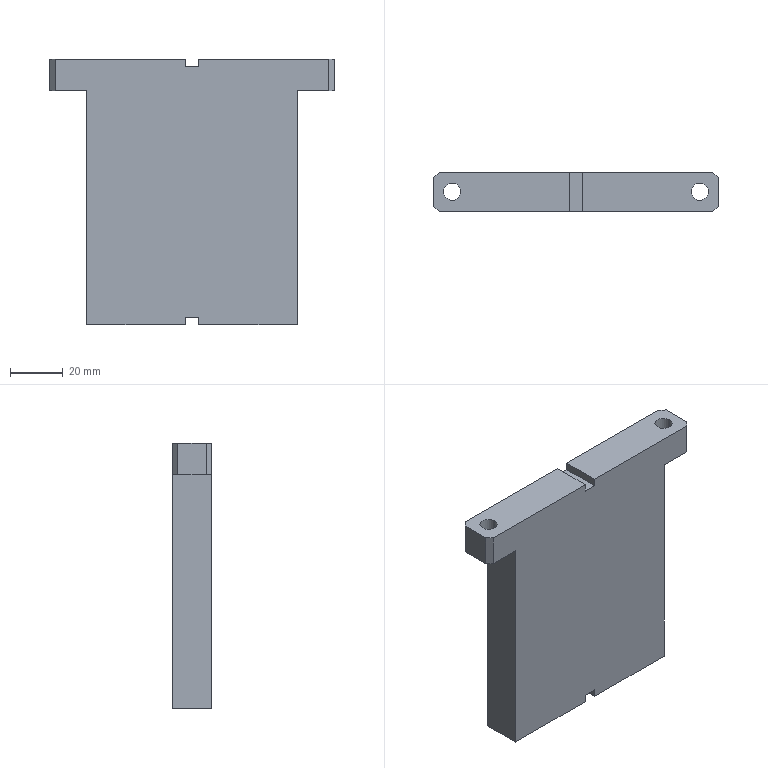Part | NX | features BREP 1 | 1 solid | 34 faces | box 108 x 15 x 101 mm | volume 124289 mm3 | plane 22 | cylinder 8 | cone 4 | commonest cylinder face diameters 5 x4 6.5 x4
STEP:
#1=CARTESIAN_POINT('',(764.522,-87.31,101.));
#2=VERTEX_POINT('',#1);
#3=CARTESIAN_POINT('',(758.022,-87.31,101.));
#4=VERTEX_POINT('',#3);
#5=CARTESIAN_POINT('',(761.272,-87.31,101.));
#6=DIRECTION('',(0.,0.,-1.));
#7=DIRECTION('',(-1.,0.,0.));
#8=AXIS2_PLACEMENT_3D('',#5,#6,#7);
#9=CIRCLE('',#8,3.25);
#10=EDGE_CURVE('',#2,#4,#9,.T.);
#11=ORIENTED_EDGE('',*,*,#10,.F.);
#12=CARTESIAN_POINT('',(764.522,-87.31,89.));
#13=VERTEX_POINT('',#12);
#14=CARTESIAN_POINT('',(764.522,-87.31,101.));
#15=DIRECTION('',(0.,0.,-1.));
#16=VECTOR('',#15,1000.);
#17=LINE('',#14,#16);
#18=EDGE_CURVE('',#2,#13,#17,.T.);
#19=ORIENTED_EDGE('',*,*,#18,.T.);
#20=CARTESIAN_POINT('',(758.022,-87.31,89.));
#21=VERTEX_POINT('',#20);
#22=CARTESIAN_POINT('',(761.272,-87.31,89.));
#23=DIRECTION('',(0.,0.,-1.));
#24=DIRECTION('',(-1.,0.,0.));
#25=AXIS2_PLACEMENT_3D('',#22,#23,#24);
#26=CIRCLE('',#25,3.25);
#27=EDGE_CURVE('',#13,#21,#26,.T.);
#28=ORIENTED_EDGE('',*,*,#27,.T.);
#29=CARTESIAN_POINT('',(758.022,-87.31,101.));
#30=DIRECTION('',(0.,0.,-1.));
#31=VECTOR('',#30,1000.);
#32=LINE('',#29,#31);
#33=EDGE_CURVE('',#4,#21,#32,.T.);
#34=ORIENTED_EDGE('',*,*,#33,.F.);
#35=EDGE_LOOP('',(#11,#19,#28,#34));
#36=FACE_BOUND('',#35,.T.);
#37=CARTESIAN_POINT('',(761.272,-87.31,101.));
#38=DIRECTION('',(0.,0.,-1.));
#39=DIRECTION('',(-1.,0.,0.));
#40=AXIS2_PLACEMENT_3D('',#37,#38,#39);
#41=CYLINDRICAL_SURFACE('',#40,3.25);
#42=ADVANCED_FACE('',(#36),#41,.F.);
#43=CARTESIAN_POINT('',(670.522,-87.31,101.));
#44=VERTEX_POINT('',#43);
#45=CARTESIAN_POINT('',(664.022,-87.31,101.));
#46=VERTEX_POINT('',#45);
#47=CARTESIAN_POINT('',(667.272,-87.31,101.));
#48=DIRECTION('',(0.,0.,-1.));
#49=DIRECTION('',(-1.,0.,0.));
#50=AXIS2_PLACEMENT_3D('',#47,#48,#49);
#51=CIRCLE('',#50,3.25);
#52=EDGE_CURVE('',#44,#46,#51,.T.);
#53=ORIENTED_EDGE('',*,*,#52,.F.);
#54=CARTESIAN_POINT('',(670.522,-87.31,89.));
#55=VERTEX_POINT('',#54);
#56=CARTESIAN_POINT('',(670.522,-87.31,101.));
#57=DIRECTION('',(0.,0.,-1.));
#58=VECTOR('',#57,1000.);
#59=LINE('',#56,#58);
#60=EDGE_CURVE('',#44,#55,#59,.T.);
#61=ORIENTED_EDGE('',*,*,#60,.T.);
#62=CARTESIAN_POINT('',(664.022,-87.31,89.));
#63=VERTEX_POINT('',#62);
#64=CARTESIAN_POINT('',(667.272,-87.31,89.));
#65=DIRECTION('',(0.,0.,-1.));
#66=DIRECTION('',(-1.,0.,0.));
#67=AXIS2_PLACEMENT_3D('',#64,#65,#66);
#68=CIRCLE('',#67,3.25);
#69=EDGE_CURVE('',#55,#63,#68,.T.);
#70=ORIENTED_EDGE('',*,*,#69,.T.);
#71=CARTESIAN_POINT('',(664.022,-87.31,101.));
#72=DIRECTION('',(0.,0.,-1.));
#73=VECTOR('',#72,1000.);
#74=LINE('',#71,#73);
#75=EDGE_CURVE('',#46,#63,#74,.T.);
#76=ORIENTED_EDGE('',*,*,#75,.F.);
#77=EDGE_LOOP('',(#53,#61,#70,#76));
#78=FACE_BOUND('',#77,.T.);
#79=CARTESIAN_POINT('',(667.272,-87.31,101.));
#80=DIRECTION('',(0.,0.,-1.));
#81=DIRECTION('',(-1.,0.,0.));
#82=AXIS2_PLACEMENT_3D('',#79,#80,#81);
#83=CYLINDRICAL_SURFACE('',#82,3.25);
#84=ADVANCED_FACE('',(#78),#83,.F.);
#85=CARTESIAN_POINT('',(689.772,-87.31,15.));
#86=VERTEX_POINT('',#85);
#87=CARTESIAN_POINT('',(684.772,-87.31,15.));
#88=VERTEX_POINT('',#87);
#89=CARTESIAN_POINT('',(687.272,-87.31,15.));
#90=DIRECTION('',(0.,0.,-1.));
#91=DIRECTION('',(-1.,0.,0.));
#92=AXIS2_PLACEMENT_3D('',#89,#90,#91);
#93=CIRCLE('',#92,2.5);
#94=EDGE_CURVE('',#86,#88,#93,.T.);
#95=ORIENTED_EDGE('',*,*,#94,.F.);
#96=CARTESIAN_POINT('',(689.772,-87.31,0.));
#97=VERTEX_POINT('',#96);
#98=CARTESIAN_POINT('',(689.772,-87.31,0.));
#99=DIRECTION('',(0.,0.,-1.));
#100=VECTOR('',#99,1000.);
#101=LINE('',#98,#100);
#102=EDGE_CURVE('',#86,#97,#101,.T.);
#103=ORIENTED_EDGE('',*,*,#102,.T.);
#104=CARTESIAN_POINT('',(684.772,-87.31,0.));
#105=VERTEX_POINT('',#104);
#106=CARTESIAN_POINT('',(687.272,-87.31,0.));
#107=DIRECTION('',(0.,0.,-1.));
#108=DIRECTION('',(-1.,0.,0.));
#109=AXIS2_PLACEMENT_3D('',#106,#107,#108);
#110=CIRCLE('',#109,2.5);
#111=EDGE_CURVE('',#97,#105,#110,.T.);
#112=ORIENTED_EDGE('',*,*,#111,.T.);
#113=CARTESIAN_POINT('',(684.772,-87.31,0.));
#114=DIRECTION('',(0.,0.,-1.));
#115=VECTOR('',#114,1000.);
#116=LINE('',#113,#115);
#117=EDGE_CURVE('',#88,#105,#116,.T.);
#118=ORIENTED_EDGE('',*,*,#117,.F.);
#119=EDGE_LOOP('',(#95,#103,#112,#118));
#120=FACE_BOUND('',#119,.T.);
#121=CARTESIAN_POINT('',(687.272,-87.31,0.));
#122=DIRECTION('',(0.,0.,-1.));
#123=DIRECTION('',(-1.,0.,0.));
#124=AXIS2_PLACEMENT_3D('',#121,#122,#123);
#125=CYLINDRICAL_SURFACE('',#124,2.5);
#126=ADVANCED_FACE('',(#120),#125,.F.);
#127=CARTESIAN_POINT('',(687.272,-87.31,16.502));
#128=VERTEX_POINT('',#127);
#129=CARTESIAN_POINT('',(684.772,-87.31,15.));
#130=DIRECTION('',(-0.8572,0.,-0.515));
#131=VECTOR('',#130,1000.);
#132=LINE('',#129,#131);
#133=EDGE_CURVE('',#128,#88,#132,.T.);
#134=ORIENTED_EDGE('',*,*,#133,.F.);
#135=CARTESIAN_POINT('',(689.772,-87.31,15.));
#136=DIRECTION('',(0.8572,0.,-0.515));
#137=VECTOR('',#136,1000.);
#138=LINE('',#135,#137);
#139=EDGE_CURVE('',#128,#86,#138,.T.);
#140=ORIENTED_EDGE('',*,*,#139,.T.);
#141=ORIENTED_EDGE('',*,*,#94,.T.);
#142=EDGE_LOOP('',(#134,#140,#141));
#143=FACE_BOUND('',#142,.T.);
#144=CARTESIAN_POINT('',(687.272,-87.31,15.));
#145=DIRECTION('',(0.,0.,-1.));
#146=DIRECTION('',(-1.,0.,0.));
#147=AXIS2_PLACEMENT_3D('',#144,#145,#146);
#148=CONICAL_SURFACE('',#147,2.5,1.03);
#149=ADVANCED_FACE('',(#143),#148,.F.);
#150=CARTESIAN_POINT('',(743.772,-87.31,15.));
#151=VERTEX_POINT('',#150);
#152=CARTESIAN_POINT('',(738.772,-87.31,15.));
#153=VERTEX_POINT('',#152);
#154=CARTESIAN_POINT('',(741.272,-87.31,15.));
#155=DIRECTION('',(0.,0.,-1.));
#156=DIRECTION('',(-1.,0.,0.));
#157=AXIS2_PLACEMENT_3D('',#154,#155,#156);
#158=CIRCLE('',#157,2.5);
#159=EDGE_CURVE('',#151,#153,#158,.T.);
#160=ORIENTED_EDGE('',*,*,#159,.F.);
#161=CARTESIAN_POINT('',(743.772,-87.31,0.));
#162=VERTEX_POINT('',#161);
#163=CARTESIAN_POINT('',(743.772,-87.31,0.));
#164=DIRECTION('',(0.,0.,-1.));
#165=VECTOR('',#164,1000.);
#166=LINE('',#163,#165);
#167=EDGE_CURVE('',#151,#162,#166,.T.);
#168=ORIENTED_EDGE('',*,*,#167,.T.);
#169=CARTESIAN_POINT('',(738.772,-87.31,0.));
#170=VERTEX_POINT('',#169);
#171=CARTESIAN_POINT('',(741.272,-87.31,0.));
#172=DIRECTION('',(0.,0.,-1.));
#173=DIRECTION('',(-1.,0.,0.));
#174=AXIS2_PLACEMENT_3D('',#171,#172,#173);
#175=CIRCLE('',#174,2.5);
#176=EDGE_CURVE('',#162,#170,#175,.T.);
#177=ORIENTED_EDGE('',*,*,#176,.T.);
#178=CARTESIAN_POINT('',(738.772,-87.31,0.));
#179=DIRECTION('',(0.,0.,-1.));
#180=VECTOR('',#179,1000.);
#181=LINE('',#178,#180);
#182=EDGE_CURVE('',#153,#170,#181,.T.);
#183=ORIENTED_EDGE('',*,*,#182,.F.);
#184=EDGE_LOOP('',(#160,#168,#177,#183));
#185=FACE_BOUND('',#184,.T.);
#186=CARTESIAN_POINT('',(741.272,-87.31,0.));
#187=DIRECTION('',(0.,0.,-1.));
#188=DIRECTION('',(-1.,0.,0.));
#189=AXIS2_PLACEMENT_3D('',#186,#187,#188);
#190=CYLINDRICAL_SURFACE('',#189,2.5);
#191=ADVANCED_FACE('',(#185),#190,.F.);
#192=CARTESIAN_POINT('',(741.272,-87.31,16.502));
#193=VERTEX_POINT('',#192);
#194=CARTESIAN_POINT('',(738.772,-87.31,15.));
#195=DIRECTION('',(-0.8572,0.,-0.515));
#196=VECTOR('',#195,1000.);
#197=LINE('',#194,#196);
#198=EDGE_CURVE('',#193,#153,#197,.T.);
#199=ORIENTED_EDGE('',*,*,#198,.F.);
#200=CARTESIAN_POINT('',(743.772,-87.31,15.));
#201=DIRECTION('',(0.8572,0.,-0.515));
#202=VECTOR('',#201,1000.);
#203=LINE('',#200,#202);
#204=EDGE_CURVE('',#193,#151,#203,.T.);
#205=ORIENTED_EDGE('',*,*,#204,.T.);
#206=ORIENTED_EDGE('',*,*,#159,.T.);
#207=EDGE_LOOP('',(#199,#205,#206));
#208=FACE_BOUND('',#207,.T.);
#209=CARTESIAN_POINT('',(741.272,-87.31,15.));
#210=DIRECTION('',(0.,0.,-1.));
#211=DIRECTION('',(-1.,0.,0.));
#212=AXIS2_PLACEMENT_3D('',#209,#210,#211);
#213=CONICAL_SURFACE('',#212,2.5,1.03);
#214=ADVANCED_FACE('',(#208),#213,.F.);
#215=CARTESIAN_POINT('',(660.272,-81.81,101.));
#216=VERTEX_POINT('',#215);
#217=CARTESIAN_POINT('',(660.272,-92.81,101.));
#218=VERTEX_POINT('',#217);
#219=CARTESIAN_POINT('',(660.272,-79.81,101.));
#220=DIRECTION('',(0.,-1.,0.));
#221=VECTOR('',#220,1000.);
#222=LINE('',#219,#221);
#223=EDGE_CURVE('',#216,#218,#222,.T.);
#224=ORIENTED_EDGE('',*,*,#223,.T.);
#225=CARTESIAN_POINT('',(662.272,-94.81,101.));
#226=VERTEX_POINT('',#225);
#227=CARTESIAN_POINT('',(660.272,-92.81,101.));
#228=DIRECTION('',(0.7071,-0.7071,0.));
#229=VECTOR('',#228,1000.);
#230=LINE('',#227,#229);
#231=EDGE_CURVE('',#218,#226,#230,.T.);
#232=ORIENTED_EDGE('',*,*,#231,.T.);
#233=CARTESIAN_POINT('',(711.772,-94.81,101.));
#234=VERTEX_POINT('',#233);
#235=CARTESIAN_POINT('',(754.272,-94.81,101.));
#236=DIRECTION('',(1.,0.,0.));
#237=VECTOR('',#236,1000.);
#238=LINE('',#235,#237);
#239=EDGE_CURVE('',#226,#234,#238,.T.);
#240=ORIENTED_EDGE('',*,*,#239,.T.);
#241=CARTESIAN_POINT('',(711.772,-79.81,101.));
#242=VERTEX_POINT('',#241);
#243=CARTESIAN_POINT('',(711.772,-94.81,101.));
#244=DIRECTION('',(0.,1.,0.));
#245=VECTOR('',#244,1000.);
#246=LINE('',#243,#245);
#247=EDGE_CURVE('',#234,#242,#246,.T.);
#248=ORIENTED_EDGE('',*,*,#247,.T.);
#249=CARTESIAN_POINT('',(662.272,-79.81,101.));
#250=VERTEX_POINT('',#249);
#251=CARTESIAN_POINT('',(754.272,-79.81,101.));
#252=DIRECTION('',(-1.,0.,0.));
#253=VECTOR('',#252,1000.);
#254=LINE('',#251,#253);
#255=EDGE_CURVE('',#242,#250,#254,.T.);
#256=ORIENTED_EDGE('',*,*,#255,.T.);
#257=CARTESIAN_POINT('',(662.272,-79.81,101.));
#258=DIRECTION('',(-0.7071,-0.7071,0.));
#259=VECTOR('',#258,1000.);
#260=LINE('',#257,#259);
#261=EDGE_CURVE('',#250,#216,#260,.T.);
#262=ORIENTED_EDGE('',*,*,#261,.T.);
#263=EDGE_LOOP('',(#224,#232,#240,#248,#256,#262));
#264=FACE_BOUND('',#263,.T.);
#265=CARTESIAN_POINT('',(667.272,-87.31,101.));
#266=DIRECTION('',(0.,0.,-1.));
#267=DIRECTION('',(-1.,0.,0.));
#268=AXIS2_PLACEMENT_3D('',#265,#266,#267);
#269=CIRCLE('',#268,3.25);
#270=EDGE_CURVE('',#46,#44,#269,.T.);
#271=ORIENTED_EDGE('',*,*,#270,.T.);
#272=ORIENTED_EDGE('',*,*,#52,.T.);
#273=EDGE_LOOP('',(#271,#272));
#274=FACE_BOUND('',#273,.T.);
#275=CARTESIAN_POINT('',(754.272,-94.81,101.));
#276=DIRECTION('',(0.,0.,-1.));
#277=DIRECTION('',(0.,-1.,0.));
#278=AXIS2_PLACEMENT_3D('',#275,#276,#277);
#279=PLANE('',#278);
#280=ADVANCED_FACE('',(#264,#274),#279,.F.);
#281=CARTESIAN_POINT('',(711.772,-94.81,0.));
#282=VERTEX_POINT('',#281);
#283=CARTESIAN_POINT('',(711.772,-79.81,0.));
#284=VERTEX_POINT('',#283);
#285=CARTESIAN_POINT('',(711.772,-79.81,0.));
#286=DIRECTION('',(0.,1.,0.));
#287=VECTOR('',#286,1000.);
#288=LINE('',#285,#287);
#289=EDGE_CURVE('',#282,#284,#288,.T.);
#290=ORIENTED_EDGE('',*,*,#289,.F.);
#291=CARTESIAN_POINT('',(674.272,-94.81,0.));
#292=VERTEX_POINT('',#291);
#293=CARTESIAN_POINT('',(754.272,-94.81,0.));
#294=DIRECTION('',(1.,0.,0.));
#295=VECTOR('',#294,1000.);
#296=LINE('',#293,#295);
#297=EDGE_CURVE('',#292,#282,#296,.T.);
#298=ORIENTED_EDGE('',*,*,#297,.F.);
#299=CARTESIAN_POINT('',(674.272,-79.81,0.));
#300=VERTEX_POINT('',#299);
#301=CARTESIAN_POINT('',(674.272,-79.81,0.));
#302=DIRECTION('',(0.,-1.,0.));
#303=VECTOR('',#302,1000.);
#304=LINE('',#301,#303);
#305=EDGE_CURVE('',#300,#292,#304,.T.);
#306=ORIENTED_EDGE('',*,*,#305,.F.);
#307=CARTESIAN_POINT('',(754.272,-79.81,0.));
#308=DIRECTION('',(-1.,0.,0.));
#309=VECTOR('',#308,1000.);
#310=LINE('',#307,#309);
#311=EDGE_CURVE('',#284,#300,#310,.T.);
#312=ORIENTED_EDGE('',*,*,#311,.F.);
#313=EDGE_LOOP('',(#290,#298,#306,#312));
#314=FACE_BOUND('',#313,.T.);
#315=CARTESIAN_POINT('',(687.272,-87.31,0.));
#316=DIRECTION('',(0.,0.,-1.));
#317=DIRECTION('',(-1.,0.,0.));
#318=AXIS2_PLACEMENT_3D('',#315,#316,#317);
#319=CIRCLE('',#318,2.5);
#320=EDGE_CURVE('',#105,#97,#319,.T.);
#321=ORIENTED_EDGE('',*,*,#320,.F.);
#322=ORIENTED_EDGE('',*,*,#111,.F.);
#323=EDGE_LOOP('',(#321,#322));
#324=FACE_BOUND('',#323,.T.);
#325=CARTESIAN_POINT('',(754.272,-94.81,0.));
#326=DIRECTION('',(0.,0.,-1.));
#327=DIRECTION('',(0.,-1.,0.));
#328=AXIS2_PLACEMENT_3D('',#325,#326,#327);
#329=PLANE('',#328);
#330=ADVANCED_FACE('',(#314,#324),#329,.T.);
#331=CARTESIAN_POINT('',(754.272,-79.81,89.));
#332=VERTEX_POINT('',#331);
#333=CARTESIAN_POINT('',(754.272,-79.81,0.));
#334=VERTEX_POINT('',#333);
#335=CARTESIAN_POINT('',(754.272,-79.81,101.));
#336=DIRECTION('',(0.,0.,-1.));
#337=VECTOR('',#336,1000.);
#338=LINE('',#335,#337);
#339=EDGE_CURVE('',#332,#334,#338,.T.);
#340=ORIENTED_EDGE('',*,*,#339,.F.);
#341=CARTESIAN_POINT('',(754.272,-94.81,89.));
#342=VERTEX_POINT('',#341);
#343=CARTESIAN_POINT('',(754.272,-79.81,89.));
#344=DIRECTION('',(0.,-1.,0.));
#345=VECTOR('',#344,1000.);
#346=LINE('',#343,#345);
#347=EDGE_CURVE('',#332,#342,#346,.T.);
#348=ORIENTED_EDGE('',*,*,#347,.T.);
#349=CARTESIAN_POINT('',(754.272,-94.81,0.));
#350=VERTEX_POINT('',#349);
#351=CARTESIAN_POINT('',(754.272,-94.81,101.));
#352=DIRECTION('',(0.,0.,-1.));
#353=VECTOR('',#352,1000.);
#354=LINE('',#351,#353);
#355=EDGE_CURVE('',#342,#350,#354,.T.);
#356=ORIENTED_EDGE('',*,*,#355,.T.);
#357=CARTESIAN_POINT('',(754.272,-79.81,0.));
#358=DIRECTION('',(0.,1.,0.));
#359=VECTOR('',#358,1000.);
#360=LINE('',#357,#359);
#361=EDGE_CURVE('',#350,#334,#360,.T.);
#362=ORIENTED_EDGE('',*,*,#361,.T.);
#363=EDGE_LOOP('',(#340,#348,#356,#362));
#364=FACE_BOUND('',#363,.T.);
#365=CARTESIAN_POINT('',(754.272,-79.81,101.));
#366=DIRECTION('',(-1.,0.,0.));
#367=DIRECTION('',(0.,0.,1.));
#368=AXIS2_PLACEMENT_3D('',#365,#366,#367);
#369=PLANE('',#368);
#370=ADVANCED_FACE('',(#364),#369,.F.);
#371=CARTESIAN_POINT('',(674.272,-79.81,89.));
#372=VERTEX_POINT('',#371);
#373=CARTESIAN_POINT('',(662.272,-79.81,89.));
#374=VERTEX_POINT('',#373);
#375=CARTESIAN_POINT('',(674.272,-79.81,89.));
#376=DIRECTION('',(-1.,0.,0.));
#377=VECTOR('',#376,1000.);
#378=LINE('',#375,#377);
#379=EDGE_CURVE('',#372,#374,#378,.T.);
#380=ORIENTED_EDGE('',*,*,#379,.T.);
#381=CARTESIAN_POINT('',(662.272,-79.81,101.));
#382=DIRECTION('',(0.,0.,1.));
#383=VECTOR('',#382,1000.);
#384=LINE('',#381,#383);
#385=EDGE_CURVE('',#374,#250,#384,.T.);
#386=ORIENTED_EDGE('',*,*,#385,.T.);
#387=ORIENTED_EDGE('',*,*,#255,.F.);
#388=CARTESIAN_POINT('',(711.772,-79.81,98.));
#389=VERTEX_POINT('',#388);
#390=CARTESIAN_POINT('',(711.772,-79.81,101.));
#391=DIRECTION('',(0.,0.,1.));
#392=VECTOR('',#391,1000.);
#393=LINE('',#390,#392);
#394=EDGE_CURVE('',#389,#242,#393,.T.);
#395=ORIENTED_EDGE('',*,*,#394,.F.);
#396=CARTESIAN_POINT('',(716.772,-79.81,98.));
#397=VERTEX_POINT('',#396);
#398=CARTESIAN_POINT('',(711.772,-79.81,98.));
#399=DIRECTION('',(-1.,0.,0.));
#400=VECTOR('',#399,1000.);
#401=LINE('',#398,#400);
#402=EDGE_CURVE('',#397,#389,#401,.T.);
#403=ORIENTED_EDGE('',*,*,#402,.F.);
#404=CARTESIAN_POINT('',(716.772,-79.81,101.));
#405=VERTEX_POINT('',#404);
#406=CARTESIAN_POINT('',(716.772,-79.81,101.));
#407=DIRECTION('',(0.,0.,-1.));
#408=VECTOR('',#407,1000.);
#409=LINE('',#406,#408);
#410=EDGE_CURVE('',#405,#397,#409,.T.);
#411=ORIENTED_EDGE('',*,*,#410,.F.);
#412=CARTESIAN_POINT('',(766.272,-79.81,101.));
#413=VERTEX_POINT('',#412);
#414=CARTESIAN_POINT('',(754.272,-79.81,101.));
#415=DIRECTION('',(-1.,0.,0.));
#416=VECTOR('',#415,1000.);
#417=LINE('',#414,#416);
#418=EDGE_CURVE('',#413,#405,#417,.T.);
#419=ORIENTED_EDGE('',*,*,#418,.F.);
#420=CARTESIAN_POINT('',(766.272,-79.81,89.));
#421=VERTEX_POINT('',#420);
#422=CARTESIAN_POINT('',(766.272,-79.81,89.));
#423=DIRECTION('',(0.,0.,-1.));
#424=VECTOR('',#423,1000.);
#425=LINE('',#422,#424);
#426=EDGE_CURVE('',#413,#421,#425,.T.);
#427=ORIENTED_EDGE('',*,*,#426,.T.);
#428=CARTESIAN_POINT('',(754.272,-79.81,89.));
#429=DIRECTION('',(-1.,0.,0.));
#430=VECTOR('',#429,1000.);
#431=LINE('',#428,#430);
#432=EDGE_CURVE('',#421,#332,#431,.T.);
#433=ORIENTED_EDGE('',*,*,#432,.T.);
#434=ORIENTED_EDGE('',*,*,#339,.T.);
#435=CARTESIAN_POINT('',(716.772,-79.81,0.));
#436=VERTEX_POINT('',#435);
#437=CARTESIAN_POINT('',(754.272,-79.81,0.));
#438=DIRECTION('',(-1.,0.,0.));
#439=VECTOR('',#438,1000.);
#440=LINE('',#437,#439);
#441=EDGE_CURVE('',#334,#436,#440,.T.);
#442=ORIENTED_EDGE('',*,*,#441,.T.);
#443=CARTESIAN_POINT('',(716.772,-79.81,3.));
#444=VERTEX_POINT('',#443);
#445=CARTESIAN_POINT('',(716.772,-79.81,3.));
#446=DIRECTION('',(0.,0.,-1.));
#447=VECTOR('',#446,1000.);
#448=LINE('',#445,#447);
#449=EDGE_CURVE('',#444,#436,#448,.T.);
#450=ORIENTED_EDGE('',*,*,#449,.F.);
#451=CARTESIAN_POINT('',(711.772,-79.81,3.));
#452=VERTEX_POINT('',#451);
#453=CARTESIAN_POINT('',(711.772,-79.81,3.));
#454=DIRECTION('',(1.,0.,0.));
#455=VECTOR('',#454,1000.);
#456=LINE('',#453,#455);
#457=EDGE_CURVE('',#452,#444,#456,.T.);
#458=ORIENTED_EDGE('',*,*,#457,.F.);
#459=CARTESIAN_POINT('',(711.772,-79.81,3.));
#460=DIRECTION('',(0.,0.,-1.));
#461=VECTOR('',#460,1000.);
#462=LINE('',#459,#461);
#463=EDGE_CURVE('',#452,#284,#462,.T.);
#464=ORIENTED_EDGE('',*,*,#463,.T.);
#465=ORIENTED_EDGE('',*,*,#311,.T.);
#466=CARTESIAN_POINT('',(674.272,-79.81,101.));
#467=DIRECTION('',(0.,0.,-1.));
#468=VECTOR('',#467,1000.);
#469=LINE('',#466,#468);
#470=EDGE_CURVE('',#372,#300,#469,.T.);
#471=ORIENTED_EDGE('',*,*,#470,.F.);
#472=EDGE_LOOP('',(#380,#386,#387,#395,#403,#411,#419,#427,#433,#434,#442,#450,#458,#464,#465,#471));
#473=FACE_BOUND('',#472,.T.);
#474=CARTESIAN_POINT('',(754.272,-79.81,101.));
#475=DIRECTION('',(0.,-1.,0.));
#476=DIRECTION('',(0.,0.,-1.));
#477=AXIS2_PLACEMENT_3D('',#474,#475,#476);
#478=PLANE('',#477);
#479=ADVANCED_FACE('',(#473),#478,.F.);
#480=CARTESIAN_POINT('',(674.272,-94.81,89.));
#481=VERTEX_POINT('',#480);
#482=CARTESIAN_POINT('',(674.272,-94.81,101.));
#483=DIRECTION('',(0.,0.,-1.));
#484=VECTOR('',#483,1000.);
#485=LINE('',#482,#484);
#486=EDGE_CURVE('',#481,#292,#485,.T.);
#487=ORIENTED_EDGE('',*,*,#486,.F.);
#488=CARTESIAN_POINT('',(674.272,-79.81,89.));
#489=DIRECTION('',(0.,1.,0.));
#490=VECTOR('',#489,1000.);
#491=LINE('',#488,#490);
#492=EDGE_CURVE('',#481,#372,#491,.T.);
#493=ORIENTED_EDGE('',*,*,#492,.T.);
#494=ORIENTED_EDGE('',*,*,#470,.T.);
#495=ORIENTED_EDGE('',*,*,#305,.T.);
#496=EDGE_LOOP('',(#487,#493,#494,#495));
#497=FACE_BOUND('',#496,.T.);
#498=CARTESIAN_POINT('',(674.272,-79.81,101.));
#499=DIRECTION('',(1.,0.,0.));
#500=DIRECTION('',(0.,-1.,0.));
#501=AXIS2_PLACEMENT_3D('',#498,#499,#500);
#502=PLANE('',#501);
#503=ADVANCED_FACE('',(#497),#502,.F.);
#504=ORIENTED_EDGE('',*,*,#239,.F.);
#505=CARTESIAN_POINT('',(662.272,-94.81,89.));
#506=VERTEX_POINT('',#505);
#507=CARTESIAN_POINT('',(662.272,-94.81,89.));
#508=DIRECTION('',(0.,0.,-1.));
#509=VECTOR('',#508,1000.);
#510=LINE('',#507,#509);
#511=EDGE_CURVE('',#226,#506,#510,.T.);
#512=ORIENTED_EDGE('',*,*,#511,.T.);
#513=CARTESIAN_POINT('',(674.272,-94.81,89.));
#514=DIRECTION('',(1.,0.,0.));
#515=VECTOR('',#514,1000.);
#516=LINE('',#513,#515);
#517=EDGE_CURVE('',#506,#481,#516,.T.);
#518=ORIENTED_EDGE('',*,*,#517,.T.);
#519=ORIENTED_EDGE('',*,*,#486,.T.);
#520=ORIENTED_EDGE('',*,*,#297,.T.);
#521=CARTESIAN_POINT('',(711.772,-94.81,3.));
#522=VERTEX_POINT('',#521);
#523=CARTESIAN_POINT('',(711.772,-94.81,3.));
#524=DIRECTION('',(0.,0.,-1.));
#525=VECTOR('',#524,1000.);
#526=LINE('',#523,#525);
#527=EDGE_CURVE('',#522,#282,#526,.T.);
#528=ORIENTED_EDGE('',*,*,#527,.F.);
#529=CARTESIAN_POINT('',(716.772,-94.81,3.));
#530=VERTEX_POINT('',#529);
#531=CARTESIAN_POINT('',(711.772,-94.81,3.));
#532=DIRECTION('',(-1.,0.,0.));
#533=VECTOR('',#532,1000.);
#534=LINE('',#531,#533);
#535=EDGE_CURVE('',#530,#522,#534,.T.);
#536=ORIENTED_EDGE('',*,*,#535,.F.);
#537=CARTESIAN_POINT('',(716.772,-94.81,0.));
#538=VERTEX_POINT('',#537);
#539=CARTESIAN_POINT('',(716.772,-94.81,3.));
#540=DIRECTION('',(0.,0.,-1.));
#541=VECTOR('',#540,1000.);
#542=LINE('',#539,#541);
#543=EDGE_CURVE('',#530,#538,#542,.T.);
#544=ORIENTED_EDGE('',*,*,#543,.T.);
#545=CARTESIAN_POINT('',(754.272,-94.81,0.));
#546=DIRECTION('',(1.,0.,0.));
#547=VECTOR('',#546,1000.);
#548=LINE('',#545,#547);
#549=EDGE_CURVE('',#538,#350,#548,.T.);
#550=ORIENTED_EDGE('',*,*,#549,.T.);
#551=ORIENTED_EDGE('',*,*,#355,.F.);
#552=CARTESIAN_POINT('',(766.272,-94.81,89.));
#553=VERTEX_POINT('',#552);
#554=CARTESIAN_POINT('',(754.272,-94.81,89.));
#555=DIRECTION('',(1.,0.,0.));
#556=VECTOR('',#555,1000.);
#557=LINE('',#554,#556);
#558=EDGE_CURVE('',#342,#553,#557,.T.);
#559=ORIENTED_EDGE('',*,*,#558,.T.);
#560=CARTESIAN_POINT('',(766.272,-94.81,101.));
#561=VERTEX_POINT('',#560);
#562=CARTESIAN_POINT('',(766.272,-94.81,101.));
#563=DIRECTION('',(0.,0.,1.));
#564=VECTOR('',#563,1000.);
#565=LINE('',#562,#564);
#566=EDGE_CURVE('',#553,#561,#565,.T.);
#567=ORIENTED_EDGE('',*,*,#566,.T.);
#568=CARTESIAN_POINT('',(716.772,-94.81,101.));
#569=VERTEX_POINT('',#568);
#570=CARTESIAN_POINT('',(754.272,-94.81,101.));
#571=DIRECTION('',(1.,0.,0.));
#572=VECTOR('',#571,1000.);
#573=LINE('',#570,#572);
#574=EDGE_CURVE('',#569,#561,#573,.T.);
#575=ORIENTED_EDGE('',*,*,#574,.F.);
#576=CARTESIAN_POINT('',(716.772,-94.81,98.));
#577=VERTEX_POINT('',#576);
#578=CARTESIAN_POINT('',(716.772,-94.81,101.));
#579=DIRECTION('',(0.,0.,-1.));
#580=VECTOR('',#579,1000.);
#581=LINE('',#578,#580);
#582=EDGE_CURVE('',#569,#577,#581,.T.);
#583=ORIENTED_EDGE('',*,*,#582,.T.);
#584=CARTESIAN_POINT('',(711.772,-94.81,98.));
#585=VERTEX_POINT('',#584);
#586=CARTESIAN_POINT('',(754.272,-94.81,98.));
#587=DIRECTION('',(-1.,0.,0.));
#588=VECTOR('',#587,1000.);
#589=LINE('',#586,#588);
#590=EDGE_CURVE('',#577,#585,#589,.T.);
#591=ORIENTED_EDGE('',*,*,#590,.T.);
#592=CARTESIAN_POINT('',(711.772,-94.81,101.));
#593=DIRECTION('',(0.,0.,1.));
#594=VECTOR('',#593,1000.);
#595=LINE('',#592,#594);
#596=EDGE_CURVE('',#585,#234,#595,.T.);
#597=ORIENTED_EDGE('',*,*,#596,.T.);
#598=EDGE_LOOP('',(#504,#512,#518,#519,#520,#528,#536,#544,#550,#551,#559,#567,#575,#583,#591,#597));
#599=FACE_BOUND('',#598,.T.);
#600=CARTESIAN_POINT('',(754.272,-94.81,101.));
#601=DIRECTION('',(0.,1.,0.));
#602=DIRECTION('',(1.,0.,0.));
#603=AXIS2_PLACEMENT_3D('',#600,#601,#602);
#604=PLANE('',#603);
#605=ADVANCED_FACE('',(#599),#604,.F.);
#606=ORIENTED_EDGE('',*,*,#574,.T.);
#607=CARTESIAN_POINT('',(768.272,-92.81,101.));
#608=VERTEX_POINT('',#607);
#609=CARTESIAN_POINT('',(766.272,-94.81,101.));
#610=DIRECTION('',(0.7071,0.7071,0.));
#611=VECTOR('',#610,1000.);
#612=LINE('',#609,#611);
#613=EDGE_CURVE('',#561,#608,#612,.T.);
#614=ORIENTED_EDGE('',*,*,#613,.T.);
#615=CARTESIAN_POINT('',(768.272,-81.81,101.));
#616=VERTEX_POINT('',#615);
#617=CARTESIAN_POINT('',(768.272,-79.81,101.));
#618=DIRECTION('',(0.,1.,0.));
#619=VECTOR('',#618,1000.);
#620=LINE('',#617,#619);
#621=EDGE_CURVE('',#608,#616,#620,.T.);
#622=ORIENTED_EDGE('',*,*,#621,.T.);
#623=CARTESIAN_POINT('',(768.272,-81.81,101.));
#624=DIRECTION('',(-0.7071,0.7071,0.));
#625=VECTOR('',#624,1000.);
#626=LINE('',#623,#625);
#627=EDGE_CURVE('',#616,#413,#626,.T.);
#628=ORIENTED_EDGE('',*,*,#627,.T.);
#629=ORIENTED_EDGE('',*,*,#418,.T.);
#630=CARTESIAN_POINT('',(716.772,-94.81,101.));
#631=DIRECTION('',(0.,-1.,0.));
#632=VECTOR('',#631,1000.);
#633=LINE('',#630,#632);
#634=EDGE_CURVE('',#405,#569,#633,.T.);
#635=ORIENTED_EDGE('',*,*,#634,.T.);
#636=EDGE_LOOP('',(#606,#614,#622,#628,#629,#635));
#637=FACE_BOUND('',#636,.T.);
#638=CARTESIAN_POINT('',(761.272,-87.31,101.));
#639=DIRECTION('',(0.,0.,-1.));
#640=DIRECTION('',(-1.,0.,0.));
#641=AXIS2_PLACEMENT_3D('',#638,#639,#640);
#642=CIRCLE('',#641,3.25);
#643=EDGE_CURVE('',#4,#2,#642,.T.);
#644=ORIENTED_EDGE('',*,*,#643,.T.);
#645=ORIENTED_EDGE('',*,*,#10,.T.);
#646=EDGE_LOOP('',(#644,#645));
#647=FACE_BOUND('',#646,.T.);
#648=CARTESIAN_POINT('',(754.272,-94.81,101.));
#649=DIRECTION('',(0.,0.,-1.));
#650=DIRECTION('',(0.,-1.,0.));
#651=AXIS2_PLACEMENT_3D('',#648,#649,#650);
#652=PLANE('',#651);
#653=ADVANCED_FACE('',(#637,#647),#652,.F.);
#654=CARTESIAN_POINT('',(716.772,-79.81,0.));
#655=DIRECTION('',(0.,-1.,0.));
#656=VECTOR('',#655,1000.);
#657=LINE('',#654,#656);
#658=EDGE_CURVE('',#436,#538,#657,.T.);
#659=ORIENTED_EDGE('',*,*,#658,.F.);
#660=ORIENTED_EDGE('',*,*,#441,.F.);
#661=ORIENTED_EDGE('',*,*,#361,.F.);
#662=ORIENTED_EDGE('',*,*,#549,.F.);
#663=EDGE_LOOP('',(#659,#660,#661,#662));
#664=FACE_BOUND('',#663,.T.);
#665=CARTESIAN_POINT('',(741.272,-87.31,0.));
#666=DIRECTION('',(0.,0.,-1.));
#667=DIRECTION('',(-1.,0.,0.));
#668=AXIS2_PLACEMENT_3D('',#665,#666,#667);
#669=CIRCLE('',#668,2.5);
#670=EDGE_CURVE('',#170,#162,#669,.T.);
#671=ORIENTED_EDGE('',*,*,#670,.F.);
#672=ORIENTED_EDGE('',*,*,#176,.F.);
#673=EDGE_LOOP('',(#671,#672));
#674=FACE_BOUND('',#673,.T.);
#675=CARTESIAN_POINT('',(754.272,-94.81,0.));
#676=DIRECTION('',(0.,0.,-1.));
#677=DIRECTION('',(0.,-1.,0.));
#678=AXIS2_PLACEMENT_3D('',#675,#676,#677);
#679=PLANE('',#678);
#680=ADVANCED_FACE('',(#664,#674),#679,.T.);
#681=ORIENTED_EDGE('',*,*,#289,.T.);
#682=ORIENTED_EDGE('',*,*,#463,.F.);
#683=CARTESIAN_POINT('',(711.772,-79.81,3.));
#684=DIRECTION('',(0.,1.,0.));
#685=VECTOR('',#684,1000.);
#686=LINE('',#683,#685);
#687=EDGE_CURVE('',#522,#452,#686,.T.);
#688=ORIENTED_EDGE('',*,*,#687,.F.);
#689=ORIENTED_EDGE('',*,*,#527,.T.);
#690=EDGE_LOOP('',(#681,#682,#688,#689));
#691=FACE_BOUND('',#690,.T.);
#692=CARTESIAN_POINT('',(711.772,-79.81,3.));
#693=DIRECTION('',(-1.,0.,0.));
#694=DIRECTION('',(0.,0.,1.));
#695=AXIS2_PLACEMENT_3D('',#692,#693,#694);
#696=PLANE('',#695);
#697=ADVANCED_FACE('',(#691),#696,.F.);
#698=ORIENTED_EDGE('',*,*,#658,.T.);
#699=ORIENTED_EDGE('',*,*,#543,.F.);
#700=CARTESIAN_POINT('',(716.772,-79.81,3.));
#701=DIRECTION('',(0.,-1.,0.));
#702=VECTOR('',#701,1000.);
#703=LINE('',#700,#702);
#704=EDGE_CURVE('',#444,#530,#703,.T.);
#705=ORIENTED_EDGE('',*,*,#704,.F.);
#706=ORIENTED_EDGE('',*,*,#449,.T.);
#707=EDGE_LOOP('',(#698,#699,#705,#706));
#708=FACE_BOUND('',#707,.T.);
#709=CARTESIAN_POINT('',(716.772,-79.81,3.));
#710=DIRECTION('',(1.,0.,0.));
#711=DIRECTION('',(0.,1.,0.));
#712=AXIS2_PLACEMENT_3D('',#709,#710,#711);
#713=PLANE('',#712);
#714=ADVANCED_FACE('',(#708),#713,.F.);
#715=ORIENTED_EDGE('',*,*,#687,.T.);
#716=ORIENTED_EDGE('',*,*,#457,.T.);
#717=ORIENTED_EDGE('',*,*,#704,.T.);
#718=ORIENTED_EDGE('',*,*,#535,.T.);
#719=EDGE_LOOP('',(#715,#716,#717,#718));
#720=FACE_BOUND('',#719,.T.);
#721=CARTESIAN_POINT('',(711.772,-94.81,3.));
#722=DIRECTION('',(0.,0.,1.));
#723=DIRECTION('',(1.,0.,0.));
#724=AXIS2_PLACEMENT_3D('',#721,#722,#723);
#725=PLANE('',#724);
#726=ADVANCED_FACE('',(#720),#725,.F.);
#727=ORIENTED_EDGE('',*,*,#204,.F.);
#728=ORIENTED_EDGE('',*,*,#198,.T.);
#729=CARTESIAN_POINT('',(741.272,-87.31,15.));
#730=DIRECTION('',(0.,0.,-1.));
#731=DIRECTION('',(-1.,0.,0.));
#732=AXIS2_PLACEMENT_3D('',#729,#730,#731);
#733=CIRCLE('',#732,2.5);
#734=EDGE_CURVE('',#153,#151,#733,.T.);
#735=ORIENTED_EDGE('',*,*,#734,.T.);
#736=EDGE_LOOP('',(#727,#728,#735));
#737=FACE_BOUND('',#736,.T.);
#738=CARTESIAN_POINT('',(741.272,-87.31,15.));
#739=DIRECTION('',(0.,0.,-1.));
#740=DIRECTION('',(-1.,0.,0.));
#741=AXIS2_PLACEMENT_3D('',#738,#739,#740);
#742=CONICAL_SURFACE('',#741,2.5,1.03);
#743=ADVANCED_FACE('',(#737),#742,.F.);
#744=ORIENTED_EDGE('',*,*,#167,.F.);
#745=ORIENTED_EDGE('',*,*,#734,.F.);
#746=ORIENTED_EDGE('',*,*,#182,.T.);
#747=ORIENTED_EDGE('',*,*,#670,.T.);
#748=EDGE_LOOP('',(#744,#745,#746,#747));
#749=FACE_BOUND('',#748,.T.);
#750=CARTESIAN_POINT('',(741.272,-87.31,0.));
#751=DIRECTION('',(0.,0.,-1.));
#752=DIRECTION('',(-1.,0.,0.));
#753=AXIS2_PLACEMENT_3D('',#750,#751,#752);
#754=CYLINDRICAL_SURFACE('',#753,2.5);
#755=ADVANCED_FACE('',(#749),#754,.F.);
#756=ORIENTED_EDGE('',*,*,#139,.F.);
#757=ORIENTED_EDGE('',*,*,#133,.T.);
#758=CARTESIAN_POINT('',(687.272,-87.31,15.));
#759=DIRECTION('',(0.,0.,-1.));
#760=DIRECTION('',(-1.,0.,0.));
#761=AXIS2_PLACEMENT_3D('',#758,#759,#760);
#762=CIRCLE('',#761,2.5);
#763=EDGE_CURVE('',#88,#86,#762,.T.);
#764=ORIENTED_EDGE('',*,*,#763,.T.);
#765=EDGE_LOOP('',(#756,#757,#764));
#766=FACE_BOUND('',#765,.T.);
#767=CARTESIAN_POINT('',(687.272,-87.31,15.));
#768=DIRECTION('',(0.,0.,-1.));
#769=DIRECTION('',(-1.,0.,0.));
#770=AXIS2_PLACEMENT_3D('',#767,#768,#769);
#771=CONICAL_SURFACE('',#770,2.5,1.03);
#772=ADVANCED_FACE('',(#766),#771,.F.);
#773=ORIENTED_EDGE('',*,*,#102,.F.);
#774=ORIENTED_EDGE('',*,*,#763,.F.);
#775=ORIENTED_EDGE('',*,*,#117,.T.);
#776=ORIENTED_EDGE('',*,*,#320,.T.);
#777=EDGE_LOOP('',(#773,#774,#775,#776));
#778=FACE_BOUND('',#777,.T.);
#779=CARTESIAN_POINT('',(687.272,-87.31,0.));
#780=DIRECTION('',(0.,0.,-1.));
#781=DIRECTION('',(-1.,0.,0.));
#782=AXIS2_PLACEMENT_3D('',#779,#780,#781);
#783=CYLINDRICAL_SURFACE('',#782,2.5);
#784=ADVANCED_FACE('',(#778),#783,.F.);
#785=ORIENTED_EDGE('',*,*,#621,.F.);
#786=CARTESIAN_POINT('',(768.272,-92.81,89.));
#787=VERTEX_POINT('',#786);
#788=CARTESIAN_POINT('',(768.272,-92.81,89.));
#789=DIRECTION('',(0.,0.,-1.));
#790=VECTOR('',#789,1000.);
#791=LINE('',#788,#790);
#792=EDGE_CURVE('',#608,#787,#791,.T.);
#793=ORIENTED_EDGE('',*,*,#792,.T.);
#794=CARTESIAN_POINT('',(768.272,-81.81,89.));
#795=VERTEX_POINT('',#794);
#796=CARTESIAN_POINT('',(768.272,-79.81,89.));
#797=DIRECTION('',(0.,1.,0.));
#798=VECTOR('',#797,1000.);
#799=LINE('',#796,#798);
#800=EDGE_CURVE('',#787,#795,#799,.T.);
#801=ORIENTED_EDGE('',*,*,#800,.T.);
#802=CARTESIAN_POINT('',(768.272,-81.81,101.));
#803=DIRECTION('',(0.,0.,1.));
#804=VECTOR('',#803,1000.);
#805=LINE('',#802,#804);
#806=EDGE_CURVE('',#795,#616,#805,.T.);
#807=ORIENTED_EDGE('',*,*,#806,.T.);
#808=EDGE_LOOP('',(#785,#793,#801,#807));
#809=FACE_BOUND('',#808,.T.);
#810=CARTESIAN_POINT('',(768.272,-79.81,89.));
#811=DIRECTION('',(1.,0.,0.));
#812=DIRECTION('',(0.,1.,0.));
#813=AXIS2_PLACEMENT_3D('',#810,#811,#812);
#814=PLANE('',#813);
#815=ADVANCED_FACE('',(#809),#814,.T.);
#816=ORIENTED_EDGE('',*,*,#800,.F.);
#817=CARTESIAN_POINT('',(766.272,-94.81,89.));
#818=DIRECTION('',(-0.7071,-0.7071,0.));
#819=VECTOR('',#818,1000.);
#820=LINE('',#817,#819);
#821=EDGE_CURVE('',#787,#553,#820,.T.);
#822=ORIENTED_EDGE('',*,*,#821,.T.);
#823=ORIENTED_EDGE('',*,*,#558,.F.);
#824=ORIENTED_EDGE('',*,*,#347,.F.);
#825=ORIENTED_EDGE('',*,*,#432,.F.);
#826=CARTESIAN_POINT('',(768.272,-81.81,89.));
#827=DIRECTION('',(0.7071,-0.7071,0.));
#828=VECTOR('',#827,1000.);
#829=LINE('',#826,#828);
#830=EDGE_CURVE('',#421,#795,#829,.T.);
#831=ORIENTED_EDGE('',*,*,#830,.T.);
#832=EDGE_LOOP('',(#816,#822,#823,#824,#825,#831));
#833=FACE_BOUND('',#832,.T.);
#834=CARTESIAN_POINT('',(761.272,-87.31,89.));
#835=DIRECTION('',(0.,0.,-1.));
#836=DIRECTION('',(-1.,0.,0.));
#837=AXIS2_PLACEMENT_3D('',#834,#835,#836);
#838=CIRCLE('',#837,3.25);
#839=EDGE_CURVE('',#21,#13,#838,.T.);
#840=ORIENTED_EDGE('',*,*,#839,.F.);
#841=ORIENTED_EDGE('',*,*,#27,.F.);
#842=EDGE_LOOP('',(#840,#841));
#843=FACE_BOUND('',#842,.T.);
#844=CARTESIAN_POINT('',(754.272,-94.81,89.));
#845=DIRECTION('',(0.,0.,1.));
#846=DIRECTION('',(1.,0.,0.));
#847=AXIS2_PLACEMENT_3D('',#844,#845,#846);
#848=PLANE('',#847);
#849=ADVANCED_FACE('',(#833,#843),#848,.F.);
#850=CARTESIAN_POINT('',(660.272,-81.81,89.));
#851=VERTEX_POINT('',#850);
#852=CARTESIAN_POINT('',(660.272,-92.81,89.));
#853=VERTEX_POINT('',#852);
#854=CARTESIAN_POINT('',(660.272,-79.81,89.));
#855=DIRECTION('',(0.,-1.,0.));
#856=VECTOR('',#855,1000.);
#857=LINE('',#854,#856);
#858=EDGE_CURVE('',#851,#853,#857,.T.);
#859=ORIENTED_EDGE('',*,*,#858,.T.);
#860=CARTESIAN_POINT('',(660.272,-92.81,101.));
#861=DIRECTION('',(0.,0.,1.));
#862=VECTOR('',#861,1000.);
#863=LINE('',#860,#862);
#864=EDGE_CURVE('',#853,#218,#863,.T.);
#865=ORIENTED_EDGE('',*,*,#864,.T.);
#866=ORIENTED_EDGE('',*,*,#223,.F.);
#867=CARTESIAN_POINT('',(660.272,-81.81,89.));
#868=DIRECTION('',(0.,0.,-1.));
#869=VECTOR('',#868,1000.);
#870=LINE('',#867,#869);
#871=EDGE_CURVE('',#216,#851,#870,.T.);
#872=ORIENTED_EDGE('',*,*,#871,.T.);
#873=EDGE_LOOP('',(#859,#865,#866,#872));
#874=FACE_BOUND('',#873,.T.);
#875=CARTESIAN_POINT('',(660.272,-79.81,89.));
#876=DIRECTION('',(-1.,0.,0.));
#877=DIRECTION('',(0.,0.,1.));
#878=AXIS2_PLACEMENT_3D('',#875,#876,#877);
#879=PLANE('',#878);
#880=ADVANCED_FACE('',(#874),#879,.T.);
#881=ORIENTED_EDGE('',*,*,#517,.F.);
#882=CARTESIAN_POINT('',(668.272,-100.81,89.));
#883=DIRECTION('',(-0.7071,0.7071,0.));
#884=VECTOR('',#883,1000.);
#885=LINE('',#882,#884);
#886=EDGE_CURVE('',#506,#853,#885,.T.);
#887=ORIENTED_EDGE('',*,*,#886,.T.);
#888=ORIENTED_EDGE('',*,*,#858,.F.);
#889=CARTESIAN_POINT('',(660.772,-81.31,89.));
#890=DIRECTION('',(0.7071,0.7071,0.));
#891=VECTOR('',#890,1000.);
#892=LINE('',#889,#891);
#893=EDGE_CURVE('',#851,#374,#892,.T.);
#894=ORIENTED_EDGE('',*,*,#893,.T.);
#895=ORIENTED_EDGE('',*,*,#379,.F.);
#896=ORIENTED_EDGE('',*,*,#492,.F.);
#897=EDGE_LOOP('',(#881,#887,#888,#894,#895,#896));
#898=FACE_BOUND('',#897,.T.);
#899=CARTESIAN_POINT('',(667.272,-87.31,89.));
#900=DIRECTION('',(0.,0.,-1.));
#901=DIRECTION('',(-1.,0.,0.));
#902=AXIS2_PLACEMENT_3D('',#899,#900,#901);
#903=CIRCLE('',#902,3.25);
#904=EDGE_CURVE('',#63,#55,#903,.T.);
#905=ORIENTED_EDGE('',*,*,#904,.F.);
#906=ORIENTED_EDGE('',*,*,#69,.F.);
#907=EDGE_LOOP('',(#905,#906));
#908=FACE_BOUND('',#907,.T.);
#909=CARTESIAN_POINT('',(674.272,-94.81,89.));
#910=DIRECTION('',(0.,0.,-1.));
#911=DIRECTION('',(0.,-1.,0.));
#912=AXIS2_PLACEMENT_3D('',#909,#910,#911);
#913=PLANE('',#912);
#914=ADVANCED_FACE('',(#898,#908),#913,.T.);
#915=ORIENTED_EDGE('',*,*,#60,.F.);
#916=ORIENTED_EDGE('',*,*,#270,.F.);
#917=ORIENTED_EDGE('',*,*,#75,.T.);
#918=ORIENTED_EDGE('',*,*,#904,.T.);
#919=EDGE_LOOP('',(#915,#916,#917,#918));
#920=FACE_BOUND('',#919,.T.);
#921=CARTESIAN_POINT('',(667.272,-87.31,101.));
#922=DIRECTION('',(0.,0.,-1.));
#923=DIRECTION('',(-1.,0.,0.));
#924=AXIS2_PLACEMENT_3D('',#921,#922,#923);
#925=CYLINDRICAL_SURFACE('',#924,3.25);
#926=ADVANCED_FACE('',(#920),#925,.F.);
#927=ORIENTED_EDGE('',*,*,#18,.F.);
#928=ORIENTED_EDGE('',*,*,#643,.F.);
#929=ORIENTED_EDGE('',*,*,#33,.T.);
#930=ORIENTED_EDGE('',*,*,#839,.T.);
#931=EDGE_LOOP('',(#927,#928,#929,#930));
#932=FACE_BOUND('',#931,.T.);
#933=CARTESIAN_POINT('',(761.272,-87.31,101.));
#934=DIRECTION('',(0.,0.,-1.));
#935=DIRECTION('',(-1.,0.,0.));
#936=AXIS2_PLACEMENT_3D('',#933,#934,#935);
#937=CYLINDRICAL_SURFACE('',#936,3.25);
#938=ADVANCED_FACE('',(#932),#937,.F.);
#939=CARTESIAN_POINT('',(716.772,-94.81,98.));
#940=DIRECTION('',(0.,1.,0.));
#941=VECTOR('',#940,1000.);
#942=LINE('',#939,#941);
#943=EDGE_CURVE('',#577,#397,#942,.T.);
#944=ORIENTED_EDGE('',*,*,#943,.T.);
#945=ORIENTED_EDGE('',*,*,#402,.T.);
#946=CARTESIAN_POINT('',(711.772,-94.81,98.));
#947=DIRECTION('',(0.,1.,0.));
#948=VECTOR('',#947,1000.);
#949=LINE('',#946,#948);
#950=EDGE_CURVE('',#585,#389,#949,.T.);
#951=ORIENTED_EDGE('',*,*,#950,.F.);
#952=ORIENTED_EDGE('',*,*,#590,.F.);
#953=EDGE_LOOP('',(#944,#945,#951,#952));
#954=FACE_BOUND('',#953,.T.);
#955=CARTESIAN_POINT('',(711.772,-94.81,98.));
#956=DIRECTION('',(0.,0.,-1.));
#957=DIRECTION('',(0.,-1.,0.));
#958=AXIS2_PLACEMENT_3D('',#955,#956,#957);
#959=PLANE('',#958);
#960=ADVANCED_FACE('',(#954),#959,.F.);
#961=ORIENTED_EDGE('',*,*,#950,.T.);
#962=ORIENTED_EDGE('',*,*,#394,.T.);
#963=ORIENTED_EDGE('',*,*,#247,.F.);
#964=ORIENTED_EDGE('',*,*,#596,.F.);
#965=EDGE_LOOP('',(#961,#962,#963,#964));
#966=FACE_BOUND('',#965,.T.);
#967=CARTESIAN_POINT('',(711.772,-94.81,101.));
#968=DIRECTION('',(-1.,0.,0.));
#969=DIRECTION('',(0.,1.,0.));
#970=AXIS2_PLACEMENT_3D('',#967,#968,#969);
#971=PLANE('',#970);
#972=ADVANCED_FACE('',(#966),#971,.F.);
#973=ORIENTED_EDGE('',*,*,#634,.F.);
#974=ORIENTED_EDGE('',*,*,#410,.T.);
#975=ORIENTED_EDGE('',*,*,#943,.F.);
#976=ORIENTED_EDGE('',*,*,#582,.F.);
#977=EDGE_LOOP('',(#973,#974,#975,#976));
#978=FACE_BOUND('',#977,.T.);
#979=CARTESIAN_POINT('',(716.772,-94.81,101.));
#980=DIRECTION('',(1.,0.,0.));
#981=DIRECTION('',(0.,1.,0.));
#982=AXIS2_PLACEMENT_3D('',#979,#980,#981);
#983=PLANE('',#982);
#984=ADVANCED_FACE('',(#978),#983,.F.);
#985=ORIENTED_EDGE('',*,*,#886,.F.);
#986=ORIENTED_EDGE('',*,*,#511,.F.);
#987=ORIENTED_EDGE('',*,*,#231,.F.);
#988=ORIENTED_EDGE('',*,*,#864,.F.);
#989=EDGE_LOOP('',(#985,#986,#987,#988));
#990=FACE_BOUND('',#989,.T.);
#991=CARTESIAN_POINT('',(660.272,-92.81,89.));
#992=DIRECTION('',(-0.7071,-0.7071,0.));
#993=DIRECTION('',(-0.7071,0.7071,0.));
#994=AXIS2_PLACEMENT_3D('',#991,#992,#993);
#995=PLANE('',#994);
#996=ADVANCED_FACE('',(#990),#995,.T.);
#997=ORIENTED_EDGE('',*,*,#893,.F.);
#998=ORIENTED_EDGE('',*,*,#871,.F.);
#999=ORIENTED_EDGE('',*,*,#261,.F.);
#1000=ORIENTED_EDGE('',*,*,#385,.F.);
#1001=EDGE_LOOP('',(#997,#998,#999,#1000));
#1002=FACE_BOUND('',#1001,.T.);
#1003=CARTESIAN_POINT('',(662.272,-79.81,101.));
#1004=DIRECTION('',(-0.7071,0.7071,0.));
#1005=DIRECTION('',(0.,0.,1.));
#1006=AXIS2_PLACEMENT_3D('',#1003,#1004,#1005);
#1007=PLANE('',#1006);
#1008=ADVANCED_FACE('',(#1002),#1007,.T.);
#1009=ORIENTED_EDGE('',*,*,#821,.F.);
#1010=ORIENTED_EDGE('',*,*,#792,.F.);
#1011=ORIENTED_EDGE('',*,*,#613,.F.);
#1012=ORIENTED_EDGE('',*,*,#566,.F.);
#1013=EDGE_LOOP('',(#1009,#1010,#1011,#1012));
#1014=FACE_BOUND('',#1013,.T.);
#1015=CARTESIAN_POINT('',(766.272,-94.81,101.));
#1016=DIRECTION('',(0.7071,-0.7071,0.));
#1017=DIRECTION('',(0.,0.,-1.));
#1018=AXIS2_PLACEMENT_3D('',#1015,#1016,#1017);
#1019=PLANE('',#1018);
#1020=ADVANCED_FACE('',(#1014),#1019,.T.);
#1021=ORIENTED_EDGE('',*,*,#830,.F.);
#1022=ORIENTED_EDGE('',*,*,#426,.F.);
#1023=ORIENTED_EDGE('',*,*,#627,.F.);
#1024=ORIENTED_EDGE('',*,*,#806,.F.);
#1025=EDGE_LOOP('',(#1021,#1022,#1023,#1024));
#1026=FACE_BOUND('',#1025,.T.);
#1027=CARTESIAN_POINT('',(768.272,-81.81,89.));
#1028=DIRECTION('',(0.7071,0.7071,0.));
#1029=DIRECTION('',(0.,0.,-1.));
#1030=AXIS2_PLACEMENT_3D('',#1027,#1028,#1029);
#1031=PLANE('',#1030);
#1032=ADVANCED_FACE('',(#1026),#1031,.T.);
#1033=CLOSED_SHELL('',(#42,#84,#126,#149,#191,#214,#280,#330,#370,#479,#503,#605,#653,#680,#697,#714,#726,#743,#755,#772,#784,#815,#849,#880,#914,#926,#938,#960,#972,#984,#996,#1008,#1020,#1032));
#1034=MANIFOLD_SOLID_BREP('',#1033);
#1035=(LENGTH_UNIT()NAMED_UNIT(*)SI_UNIT(.MILLI.,.METRE.));
#1036=UNCERTAINTY_MEASURE_WITH_UNIT(LENGTH_MEASURE(0.00001),#1035,'','');
#1037=(NAMED_UNIT(*)PLANE_ANGLE_UNIT()SI_UNIT($,.RADIAN.));
#1038=(NAMED_UNIT(*)SI_UNIT($,.STERADIAN.)SOLID_ANGLE_UNIT());
#1039=(GEOMETRIC_REPRESENTATION_CONTEXT(3)GLOBAL_UNCERTAINTY_ASSIGNED_CONTEXT((#1036))GLOBAL_UNIT_ASSIGNED_CONTEXT((#1035,#1037,#1038))REPRESENTATION_CONTEXT('',''));
#1040=ADVANCED_BREP_SHAPE_REPRESENTATION('',(#1034),#1039);